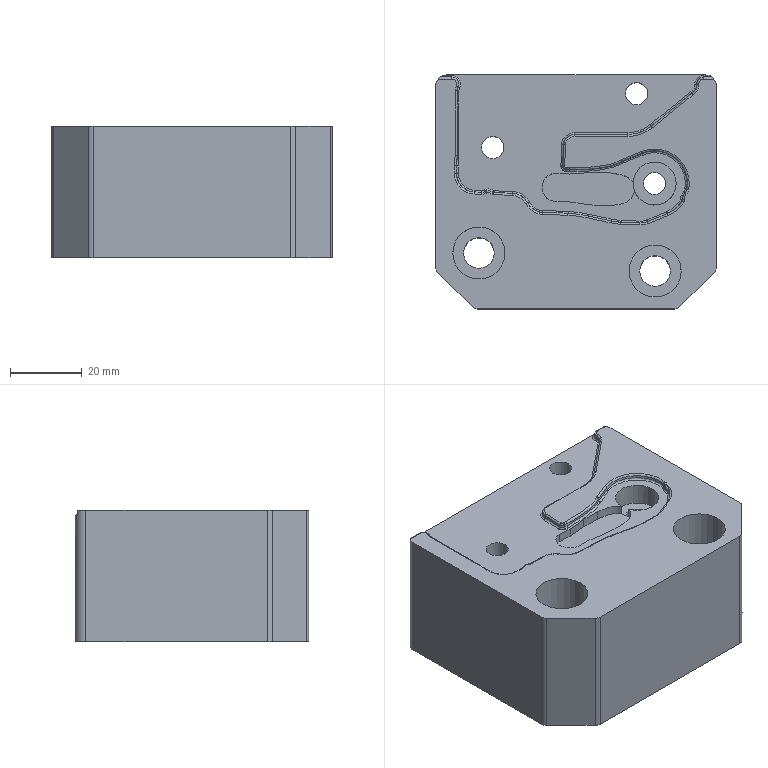Part | NX | features DIE-42 2 | 1 solid | 164 faces | box 78 x 65 x 36.5 mm | volume 166808 mm3 | spline 86 | cylinder 44 | plane 28 | torus 4 | cone 2 | commonest cylinder face diameters 1 x30 4 x4 6.201 x3 6 x2 8.506 x2 14.5 x2